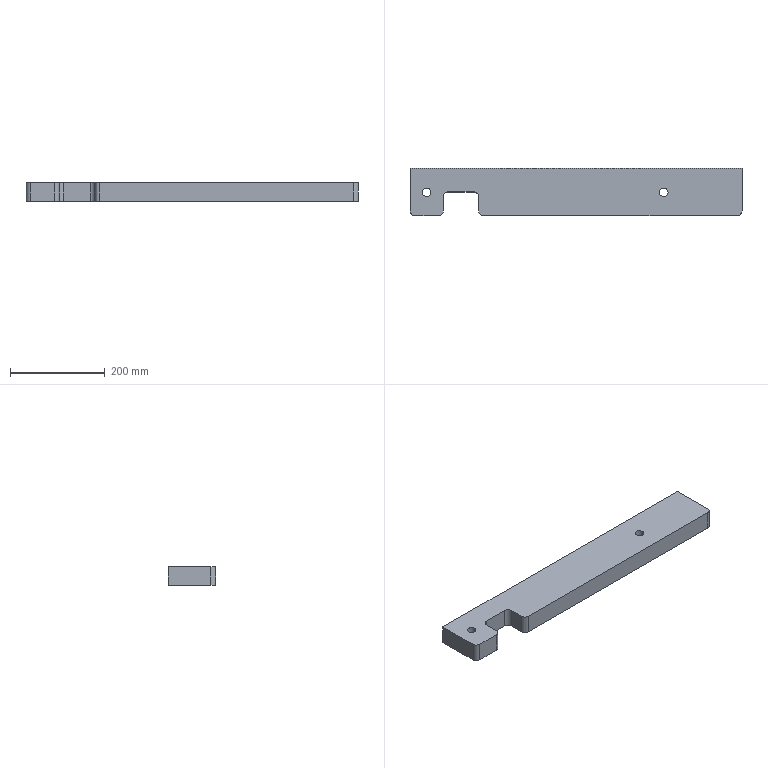Part | SolidWorks | features Extrusion 1, Fillet 1 | 1 solid | 20 faces | box 700 x 100 x 40 mm | volume 2627926 mm3 | cylinder 10 | plane 10 | commonest cylinder face diameters 20 x6 18 x4
STEP:
#1=CARTESIAN_POINT('',(526.,49.,40.));
#2=VERTEX_POINT('',#1);
#3=CARTESIAN_POINT('',(544.,49.,40.));
#4=VERTEX_POINT('',#3);
#5=CARTESIAN_POINT('',(535.,49.,40.));
#6=DIRECTION('',(0.,0.,1.));
#7=DIRECTION('',(1.,0.,0.));
#8=AXIS2_PLACEMENT_3D('',#5,#6,#7);
#9=CIRCLE('',#8,9.);
#10=EDGE_CURVE('',#2,#4,#9,.T.);
#11=ORIENTED_EDGE('',*,*,#10,.T.);
#12=CARTESIAN_POINT('',(544.,49.,0.));
#13=VERTEX_POINT('',#12);
#14=CARTESIAN_POINT('',(544.,49.,40.));
#15=DIRECTION('',(0.,0.,-1.));
#16=VECTOR('',#15,1000.);
#17=LINE('',#14,#16);
#18=EDGE_CURVE('',#4,#13,#17,.T.);
#19=ORIENTED_EDGE('',*,*,#18,.T.);
#20=CARTESIAN_POINT('',(526.,49.,0.));
#21=VERTEX_POINT('',#20);
#22=CARTESIAN_POINT('',(535.,49.,0.));
#23=DIRECTION('',(0.,0.,1.));
#24=DIRECTION('',(1.,0.,0.));
#25=AXIS2_PLACEMENT_3D('',#22,#23,#24);
#26=CIRCLE('',#25,9.);
#27=EDGE_CURVE('',#21,#13,#26,.T.);
#28=ORIENTED_EDGE('',*,*,#27,.F.);
#29=CARTESIAN_POINT('',(526.,49.,40.));
#30=DIRECTION('',(0.,0.,-1.));
#31=VECTOR('',#30,1000.);
#32=LINE('',#29,#31);
#33=EDGE_CURVE('',#2,#21,#32,.T.);
#34=ORIENTED_EDGE('',*,*,#33,.F.);
#35=EDGE_LOOP('',(#11,#19,#28,#34));
#36=FACE_OUTER_BOUND('',#35,.T.);
#37=CARTESIAN_POINT('',(535.,49.,40.));
#38=DIRECTION('',(0.,0.,-1.));
#39=DIRECTION('',(-1.,0.,0.));
#40=AXIS2_PLACEMENT_3D('',#37,#38,#39);
#41=CYLINDRICAL_SURFACE('',#40,9.);
#42=ADVANCED_FACE('',(#36),#41,.F.);
#43=CARTESIAN_POINT('',(26.,49.,40.));
#44=VERTEX_POINT('',#43);
#45=CARTESIAN_POINT('',(44.,49.,40.));
#46=VERTEX_POINT('',#45);
#47=CARTESIAN_POINT('',(35.,49.,40.));
#48=DIRECTION('',(0.,0.,1.));
#49=DIRECTION('',(1.,0.,0.));
#50=AXIS2_PLACEMENT_3D('',#47,#48,#49);
#51=CIRCLE('',#50,9.);
#52=EDGE_CURVE('',#44,#46,#51,.T.);
#53=ORIENTED_EDGE('',*,*,#52,.T.);
#54=CARTESIAN_POINT('',(44.,49.,0.));
#55=VERTEX_POINT('',#54);
#56=CARTESIAN_POINT('',(44.,49.,40.));
#57=DIRECTION('',(0.,0.,-1.));
#58=VECTOR('',#57,1000.);
#59=LINE('',#56,#58);
#60=EDGE_CURVE('',#46,#55,#59,.T.);
#61=ORIENTED_EDGE('',*,*,#60,.T.);
#62=CARTESIAN_POINT('',(26.,49.,0.));
#63=VERTEX_POINT('',#62);
#64=CARTESIAN_POINT('',(35.,49.,0.));
#65=DIRECTION('',(0.,0.,1.));
#66=DIRECTION('',(1.,0.,0.));
#67=AXIS2_PLACEMENT_3D('',#64,#65,#66);
#68=CIRCLE('',#67,9.);
#69=EDGE_CURVE('',#63,#55,#68,.T.);
#70=ORIENTED_EDGE('',*,*,#69,.F.);
#71=CARTESIAN_POINT('',(26.,49.,40.));
#72=DIRECTION('',(0.,0.,-1.));
#73=VECTOR('',#72,1000.);
#74=LINE('',#71,#73);
#75=EDGE_CURVE('',#44,#63,#74,.T.);
#76=ORIENTED_EDGE('',*,*,#75,.F.);
#77=EDGE_LOOP('',(#53,#61,#70,#76));
#78=FACE_OUTER_BOUND('',#77,.T.);
#79=CARTESIAN_POINT('',(35.,49.,40.));
#80=DIRECTION('',(0.,0.,-1.));
#81=DIRECTION('',(-1.,0.,0.));
#82=AXIS2_PLACEMENT_3D('',#79,#80,#81);
#83=CYLINDRICAL_SURFACE('',#82,9.);
#84=ADVANCED_FACE('',(#78),#83,.F.);
#85=ORIENTED_EDGE('',*,*,#52,.F.);
#86=CARTESIAN_POINT('',(35.,49.,40.));
#87=DIRECTION('',(0.,0.,1.));
#88=DIRECTION('',(1.,0.,0.));
#89=AXIS2_PLACEMENT_3D('',#86,#87,#88);
#90=CIRCLE('',#89,9.);
#91=EDGE_CURVE('',#46,#44,#90,.T.);
#92=ORIENTED_EDGE('',*,*,#91,.F.);
#93=EDGE_LOOP('',(#85,#92));
#94=FACE_BOUND('',#93,.T.);
#95=CARTESIAN_POINT('',(155.,0.,40.));
#96=VERTEX_POINT('',#95);
#97=CARTESIAN_POINT('',(690.,0.,40.));
#98=VERTEX_POINT('',#97);
#99=CARTESIAN_POINT('',(700.,0.,40.));
#100=DIRECTION('',(1.,0.,0.));
#101=VECTOR('',#100,1000.);
#102=LINE('',#99,#101);
#103=EDGE_CURVE('',#96,#98,#102,.T.);
#104=ORIENTED_EDGE('',*,*,#103,.T.);
#105=CARTESIAN_POINT('',(700.,10.,40.));
#106=VERTEX_POINT('',#105);
#107=CARTESIAN_POINT('',(690.,10.,40.));
#108=DIRECTION('',(0.,0.,1.));
#109=DIRECTION('',(1.,0.,0.));
#110=AXIS2_PLACEMENT_3D('',#107,#108,#109);
#111=CIRCLE('',#110,10.);
#112=EDGE_CURVE('',#98,#106,#111,.T.);
#113=ORIENTED_EDGE('',*,*,#112,.T.);
#114=CARTESIAN_POINT('',(700.,100.,40.));
#115=VERTEX_POINT('',#114);
#116=CARTESIAN_POINT('',(700.,0.,40.));
#117=DIRECTION('',(0.,1.,0.));
#118=VECTOR('',#117,1000.);
#119=LINE('',#116,#118);
#120=EDGE_CURVE('',#106,#115,#119,.T.);
#121=ORIENTED_EDGE('',*,*,#120,.T.);
#122=CARTESIAN_POINT('',(0.,100.,40.));
#123=VERTEX_POINT('',#122);
#124=CARTESIAN_POINT('',(0.,100.,40.));
#125=DIRECTION('',(-1.,0.,0.));
#126=VECTOR('',#125,1000.);
#127=LINE('',#124,#126);
#128=EDGE_CURVE('',#115,#123,#127,.T.);
#129=ORIENTED_EDGE('',*,*,#128,.T.);
#130=CARTESIAN_POINT('',(0.,10.,40.));
#131=VERTEX_POINT('',#130);
#132=CARTESIAN_POINT('',(0.,0.,40.));
#133=DIRECTION('',(0.,-1.,0.));
#134=VECTOR('',#133,1000.);
#135=LINE('',#132,#134);
#136=EDGE_CURVE('',#123,#131,#135,.T.);
#137=ORIENTED_EDGE('',*,*,#136,.T.);
#138=CARTESIAN_POINT('',(10.,0.,40.));
#139=VERTEX_POINT('',#138);
#140=CARTESIAN_POINT('',(10.,10.,40.));
#141=DIRECTION('',(0.,0.,1.));
#142=DIRECTION('',(1.,0.,0.));
#143=AXIS2_PLACEMENT_3D('',#140,#141,#142);
#144=CIRCLE('',#143,10.);
#145=EDGE_CURVE('',#131,#139,#144,.T.);
#146=ORIENTED_EDGE('',*,*,#145,.T.);
#147=CARTESIAN_POINT('',(60.,0.,40.));
#148=VERTEX_POINT('',#147);
#149=CARTESIAN_POINT('',(70.,0.,40.));
#150=DIRECTION('',(1.,0.,0.));
#151=VECTOR('',#150,1000.);
#152=LINE('',#149,#151);
#153=EDGE_CURVE('',#139,#148,#152,.T.);
#154=ORIENTED_EDGE('',*,*,#153,.T.);
#155=CARTESIAN_POINT('',(70.,10.,40.));
#156=VERTEX_POINT('',#155);
#157=CARTESIAN_POINT('',(60.,10.,40.));
#158=DIRECTION('',(0.,0.,1.));
#159=DIRECTION('',(1.,0.,0.));
#160=AXIS2_PLACEMENT_3D('',#157,#158,#159);
#161=CIRCLE('',#160,10.);
#162=EDGE_CURVE('',#148,#156,#161,.T.);
#163=ORIENTED_EDGE('',*,*,#162,.T.);
#164=CARTESIAN_POINT('',(70.,40.,40.));
#165=VERTEX_POINT('',#164);
#166=CARTESIAN_POINT('',(70.,0.,40.));
#167=DIRECTION('',(0.,1.,0.));
#168=VECTOR('',#167,1000.);
#169=LINE('',#166,#168);
#170=EDGE_CURVE('',#156,#165,#169,.T.);
#171=ORIENTED_EDGE('',*,*,#170,.T.);
#172=CARTESIAN_POINT('',(80.,50.,40.));
#173=VERTEX_POINT('',#172);
#174=CARTESIAN_POINT('',(80.,40.,40.));
#175=DIRECTION('',(0.,0.,-1.));
#176=DIRECTION('',(1.,0.,0.));
#177=AXIS2_PLACEMENT_3D('',#174,#175,#176);
#178=CIRCLE('',#177,10.);
#179=EDGE_CURVE('',#165,#173,#178,.T.);
#180=ORIENTED_EDGE('',*,*,#179,.T.);
#181=CARTESIAN_POINT('',(135.,50.,40.));
#182=VERTEX_POINT('',#181);
#183=CARTESIAN_POINT('',(70.,50.,40.));
#184=DIRECTION('',(1.,0.,0.));
#185=VECTOR('',#184,1000.);
#186=LINE('',#183,#185);
#187=EDGE_CURVE('',#173,#182,#186,.T.);
#188=ORIENTED_EDGE('',*,*,#187,.T.);
#189=CARTESIAN_POINT('',(145.,40.,40.));
#190=VERTEX_POINT('',#189);
#191=CARTESIAN_POINT('',(135.,40.,40.));
#192=DIRECTION('',(0.,0.,-1.));
#193=DIRECTION('',(1.,0.,0.));
#194=AXIS2_PLACEMENT_3D('',#191,#192,#193);
#195=CIRCLE('',#194,10.);
#196=EDGE_CURVE('',#182,#190,#195,.T.);
#197=ORIENTED_EDGE('',*,*,#196,.T.);
#198=CARTESIAN_POINT('',(145.,10.,40.));
#199=VERTEX_POINT('',#198);
#200=CARTESIAN_POINT('',(145.,50.,40.));
#201=DIRECTION('',(0.,-1.,0.));
#202=VECTOR('',#201,1000.);
#203=LINE('',#200,#202);
#204=EDGE_CURVE('',#190,#199,#203,.T.);
#205=ORIENTED_EDGE('',*,*,#204,.T.);
#206=CARTESIAN_POINT('',(155.,10.,40.));
#207=DIRECTION('',(0.,0.,1.));
#208=DIRECTION('',(1.,0.,0.));
#209=AXIS2_PLACEMENT_3D('',#206,#207,#208);
#210=CIRCLE('',#209,10.);
#211=EDGE_CURVE('',#199,#96,#210,.T.);
#212=ORIENTED_EDGE('',*,*,#211,.T.);
#213=EDGE_LOOP('',(#104,#113,#121,#129,#137,#146,#154,#163,#171,#180,#188,#197,#205,#212));
#214=FACE_OUTER_BOUND('',#213,.T.);
#215=ORIENTED_EDGE('',*,*,#10,.F.);
#216=CARTESIAN_POINT('',(535.,49.,40.));
#217=DIRECTION('',(0.,0.,1.));
#218=DIRECTION('',(1.,0.,0.));
#219=AXIS2_PLACEMENT_3D('',#216,#217,#218);
#220=CIRCLE('',#219,9.);
#221=EDGE_CURVE('',#4,#2,#220,.T.);
#222=ORIENTED_EDGE('',*,*,#221,.F.);
#223=EDGE_LOOP('',(#215,#222));
#224=FACE_BOUND('',#223,.T.);
#225=CARTESIAN_POINT('',(0.,0.,40.));
#226=DIRECTION('',(0.,0.,1.));
#227=DIRECTION('',(1.,0.,0.));
#228=AXIS2_PLACEMENT_3D('',#225,#226,#227);
#229=PLANE('',#228);
#230=ADVANCED_FACE('',(#94,#214,#224),#229,.T.);
#231=CARTESIAN_POINT('',(700.,10.,0.));
#232=VERTEX_POINT('',#231);
#233=CARTESIAN_POINT('',(700.,100.,0.));
#234=VERTEX_POINT('',#233);
#235=CARTESIAN_POINT('',(700.,0.,0.));
#236=DIRECTION('',(0.,1.,0.));
#237=VECTOR('',#236,1000.);
#238=LINE('',#235,#237);
#239=EDGE_CURVE('',#232,#234,#238,.T.);
#240=ORIENTED_EDGE('',*,*,#239,.F.);
#241=CARTESIAN_POINT('',(690.,0.,0.));
#242=VERTEX_POINT('',#241);
#243=CARTESIAN_POINT('',(690.,10.,0.));
#244=DIRECTION('',(0.,0.,-1.));
#245=DIRECTION('',(1.,0.,0.));
#246=AXIS2_PLACEMENT_3D('',#243,#244,#245);
#247=CIRCLE('',#246,10.);
#248=EDGE_CURVE('',#232,#242,#247,.T.);
#249=ORIENTED_EDGE('',*,*,#248,.T.);
#250=CARTESIAN_POINT('',(155.,0.,0.));
#251=VERTEX_POINT('',#250);
#252=CARTESIAN_POINT('',(700.,0.,0.));
#253=DIRECTION('',(1.,0.,0.));
#254=VECTOR('',#253,1000.);
#255=LINE('',#252,#254);
#256=EDGE_CURVE('',#251,#242,#255,.T.);
#257=ORIENTED_EDGE('',*,*,#256,.F.);
#258=CARTESIAN_POINT('',(145.,10.,0.));
#259=VERTEX_POINT('',#258);
#260=CARTESIAN_POINT('',(155.,10.,0.));
#261=DIRECTION('',(0.,0.,-1.));
#262=DIRECTION('',(1.,0.,0.));
#263=AXIS2_PLACEMENT_3D('',#260,#261,#262);
#264=CIRCLE('',#263,10.);
#265=EDGE_CURVE('',#251,#259,#264,.T.);
#266=ORIENTED_EDGE('',*,*,#265,.T.);
#267=CARTESIAN_POINT('',(145.,40.,0.));
#268=VERTEX_POINT('',#267);
#269=CARTESIAN_POINT('',(145.,50.,0.));
#270=DIRECTION('',(0.,-1.,0.));
#271=VECTOR('',#270,1000.);
#272=LINE('',#269,#271);
#273=EDGE_CURVE('',#268,#259,#272,.T.);
#274=ORIENTED_EDGE('',*,*,#273,.F.);
#275=CARTESIAN_POINT('',(135.,50.,0.));
#276=VERTEX_POINT('',#275);
#277=CARTESIAN_POINT('',(135.,40.,0.));
#278=DIRECTION('',(0.,0.,1.));
#279=DIRECTION('',(1.,0.,0.));
#280=AXIS2_PLACEMENT_3D('',#277,#278,#279);
#281=CIRCLE('',#280,10.);
#282=EDGE_CURVE('',#268,#276,#281,.T.);
#283=ORIENTED_EDGE('',*,*,#282,.T.);
#284=CARTESIAN_POINT('',(80.,50.,0.));
#285=VERTEX_POINT('',#284);
#286=CARTESIAN_POINT('',(70.,50.,0.));
#287=DIRECTION('',(1.,0.,0.));
#288=VECTOR('',#287,1000.);
#289=LINE('',#286,#288);
#290=EDGE_CURVE('',#285,#276,#289,.T.);
#291=ORIENTED_EDGE('',*,*,#290,.F.);
#292=CARTESIAN_POINT('',(70.,40.,0.));
#293=VERTEX_POINT('',#292);
#294=CARTESIAN_POINT('',(80.,40.,0.));
#295=DIRECTION('',(0.,0.,1.));
#296=DIRECTION('',(1.,0.,0.));
#297=AXIS2_PLACEMENT_3D('',#294,#295,#296);
#298=CIRCLE('',#297,10.);
#299=EDGE_CURVE('',#285,#293,#298,.T.);
#300=ORIENTED_EDGE('',*,*,#299,.T.);
#301=CARTESIAN_POINT('',(70.,10.,0.));
#302=VERTEX_POINT('',#301);
#303=CARTESIAN_POINT('',(70.,0.,0.));
#304=DIRECTION('',(0.,1.,0.));
#305=VECTOR('',#304,1000.);
#306=LINE('',#303,#305);
#307=EDGE_CURVE('',#302,#293,#306,.T.);
#308=ORIENTED_EDGE('',*,*,#307,.F.);
#309=CARTESIAN_POINT('',(60.,0.,0.));
#310=VERTEX_POINT('',#309);
#311=CARTESIAN_POINT('',(60.,10.,0.));
#312=DIRECTION('',(0.,0.,-1.));
#313=DIRECTION('',(1.,0.,0.));
#314=AXIS2_PLACEMENT_3D('',#311,#312,#313);
#315=CIRCLE('',#314,10.);
#316=EDGE_CURVE('',#302,#310,#315,.T.);
#317=ORIENTED_EDGE('',*,*,#316,.T.);
#318=CARTESIAN_POINT('',(10.,0.,0.));
#319=VERTEX_POINT('',#318);
#320=CARTESIAN_POINT('',(70.,0.,0.));
#321=DIRECTION('',(1.,0.,0.));
#322=VECTOR('',#321,1000.);
#323=LINE('',#320,#322);
#324=EDGE_CURVE('',#319,#310,#323,.T.);
#325=ORIENTED_EDGE('',*,*,#324,.F.);
#326=CARTESIAN_POINT('',(0.,10.,0.));
#327=VERTEX_POINT('',#326);
#328=CARTESIAN_POINT('',(10.,10.,0.));
#329=DIRECTION('',(0.,0.,-1.));
#330=DIRECTION('',(1.,0.,0.));
#331=AXIS2_PLACEMENT_3D('',#328,#329,#330);
#332=CIRCLE('',#331,10.);
#333=EDGE_CURVE('',#319,#327,#332,.T.);
#334=ORIENTED_EDGE('',*,*,#333,.T.);
#335=CARTESIAN_POINT('',(0.,100.,0.));
#336=VERTEX_POINT('',#335);
#337=CARTESIAN_POINT('',(0.,0.,0.));
#338=DIRECTION('',(0.,-1.,0.));
#339=VECTOR('',#338,1000.);
#340=LINE('',#337,#339);
#341=EDGE_CURVE('',#336,#327,#340,.T.);
#342=ORIENTED_EDGE('',*,*,#341,.F.);
#343=CARTESIAN_POINT('',(0.,100.,0.));
#344=DIRECTION('',(-1.,0.,0.));
#345=VECTOR('',#344,1000.);
#346=LINE('',#343,#345);
#347=EDGE_CURVE('',#234,#336,#346,.T.);
#348=ORIENTED_EDGE('',*,*,#347,.F.);
#349=EDGE_LOOP('',(#240,#249,#257,#266,#274,#283,#291,#300,#308,#317,#325,#334,#342,#348));
#350=FACE_OUTER_BOUND('',#349,.T.);
#351=ORIENTED_EDGE('',*,*,#69,.T.);
#352=CARTESIAN_POINT('',(35.,49.,0.));
#353=DIRECTION('',(0.,0.,1.));
#354=DIRECTION('',(1.,0.,0.));
#355=AXIS2_PLACEMENT_3D('',#352,#353,#354);
#356=CIRCLE('',#355,9.);
#357=EDGE_CURVE('',#55,#63,#356,.T.);
#358=ORIENTED_EDGE('',*,*,#357,.T.);
#359=EDGE_LOOP('',(#351,#358));
#360=FACE_BOUND('',#359,.T.);
#361=ORIENTED_EDGE('',*,*,#27,.T.);
#362=CARTESIAN_POINT('',(535.,49.,0.));
#363=DIRECTION('',(0.,0.,1.));
#364=DIRECTION('',(1.,0.,0.));
#365=AXIS2_PLACEMENT_3D('',#362,#363,#364);
#366=CIRCLE('',#365,9.);
#367=EDGE_CURVE('',#13,#21,#366,.T.);
#368=ORIENTED_EDGE('',*,*,#367,.T.);
#369=EDGE_LOOP('',(#361,#368));
#370=FACE_BOUND('',#369,.T.);
#371=CARTESIAN_POINT('',(0.,0.,0.));
#372=DIRECTION('',(0.,0.,1.));
#373=DIRECTION('',(1.,0.,0.));
#374=AXIS2_PLACEMENT_3D('',#371,#372,#373);
#375=PLANE('',#374);
#376=ADVANCED_FACE('',(#350,#360,#370),#375,.F.);
#377=ORIENTED_EDGE('',*,*,#256,.T.);
#378=CARTESIAN_POINT('',(690.,0.,40.));
#379=DIRECTION('',(0.,0.,1.));
#380=VECTOR('',#379,1000.);
#381=LINE('',#378,#380);
#382=EDGE_CURVE('',#242,#98,#381,.T.);
#383=ORIENTED_EDGE('',*,*,#382,.T.);
#384=ORIENTED_EDGE('',*,*,#103,.F.);
#385=CARTESIAN_POINT('',(155.,0.,40.));
#386=DIRECTION('',(0.,0.,-1.));
#387=VECTOR('',#386,1000.);
#388=LINE('',#385,#387);
#389=EDGE_CURVE('',#96,#251,#388,.T.);
#390=ORIENTED_EDGE('',*,*,#389,.T.);
#391=EDGE_LOOP('',(#377,#383,#384,#390));
#392=FACE_OUTER_BOUND('',#391,.T.);
#393=CARTESIAN_POINT('',(700.,0.,40.));
#394=DIRECTION('',(0.,1.,0.));
#395=DIRECTION('',(-1.,0.,0.));
#396=AXIS2_PLACEMENT_3D('',#393,#394,#395);
#397=PLANE('',#396);
#398=ADVANCED_FACE('',(#392),#397,.F.);
#399=ORIENTED_EDGE('',*,*,#120,.F.);
#400=CARTESIAN_POINT('',(700.,10.,40.));
#401=DIRECTION('',(0.,0.,-1.));
#402=VECTOR('',#401,1000.);
#403=LINE('',#400,#402);
#404=EDGE_CURVE('',#106,#232,#403,.T.);
#405=ORIENTED_EDGE('',*,*,#404,.T.);
#406=ORIENTED_EDGE('',*,*,#239,.T.);
#407=CARTESIAN_POINT('',(700.,100.,40.));
#408=DIRECTION('',(0.,0.,-1.));
#409=VECTOR('',#408,1000.);
#410=LINE('',#407,#409);
#411=EDGE_CURVE('',#115,#234,#410,.T.);
#412=ORIENTED_EDGE('',*,*,#411,.F.);
#413=EDGE_LOOP('',(#399,#405,#406,#412));
#414=FACE_OUTER_BOUND('',#413,.T.);
#415=CARTESIAN_POINT('',(700.,0.,40.));
#416=DIRECTION('',(-1.,0.,0.));
#417=DIRECTION('',(0.,0.,1.));
#418=AXIS2_PLACEMENT_3D('',#415,#416,#417);
#419=PLANE('',#418);
#420=ADVANCED_FACE('',(#414),#419,.F.);
#421=ORIENTED_EDGE('',*,*,#347,.T.);
#422=CARTESIAN_POINT('',(0.,100.,40.));
#423=DIRECTION('',(0.,0.,-1.));
#424=VECTOR('',#423,1000.);
#425=LINE('',#422,#424);
#426=EDGE_CURVE('',#123,#336,#425,.T.);
#427=ORIENTED_EDGE('',*,*,#426,.F.);
#428=ORIENTED_EDGE('',*,*,#128,.F.);
#429=ORIENTED_EDGE('',*,*,#411,.T.);
#430=EDGE_LOOP('',(#421,#427,#428,#429));
#431=FACE_OUTER_BOUND('',#430,.T.);
#432=CARTESIAN_POINT('',(0.,100.,40.));
#433=DIRECTION('',(0.,-1.,0.));
#434=DIRECTION('',(1.,0.,0.));
#435=AXIS2_PLACEMENT_3D('',#432,#433,#434);
#436=PLANE('',#435);
#437=ADVANCED_FACE('',(#431),#436,.F.);
#438=ORIENTED_EDGE('',*,*,#341,.T.);
#439=CARTESIAN_POINT('',(0.,10.,40.));
#440=DIRECTION('',(0.,0.,1.));
#441=VECTOR('',#440,1000.);
#442=LINE('',#439,#441);
#443=EDGE_CURVE('',#327,#131,#442,.T.);
#444=ORIENTED_EDGE('',*,*,#443,.T.);
#445=ORIENTED_EDGE('',*,*,#136,.F.);
#446=ORIENTED_EDGE('',*,*,#426,.T.);
#447=EDGE_LOOP('',(#438,#444,#445,#446));
#448=FACE_OUTER_BOUND('',#447,.T.);
#449=CARTESIAN_POINT('',(0.,0.,40.));
#450=DIRECTION('',(1.,0.,0.));
#451=DIRECTION('',(0.,0.,-1.));
#452=AXIS2_PLACEMENT_3D('',#449,#450,#451);
#453=PLANE('',#452);
#454=ADVANCED_FACE('',(#448),#453,.F.);
#455=ORIENTED_EDGE('',*,*,#153,.F.);
#456=CARTESIAN_POINT('',(10.,0.,40.));
#457=DIRECTION('',(0.,0.,-1.));
#458=VECTOR('',#457,1000.);
#459=LINE('',#456,#458);
#460=EDGE_CURVE('',#139,#319,#459,.T.);
#461=ORIENTED_EDGE('',*,*,#460,.T.);
#462=ORIENTED_EDGE('',*,*,#324,.T.);
#463=CARTESIAN_POINT('',(60.,0.,40.));
#464=DIRECTION('',(0.,0.,1.));
#465=VECTOR('',#464,1000.);
#466=LINE('',#463,#465);
#467=EDGE_CURVE('',#310,#148,#466,.T.);
#468=ORIENTED_EDGE('',*,*,#467,.T.);
#469=EDGE_LOOP('',(#455,#461,#462,#468));
#470=FACE_OUTER_BOUND('',#469,.T.);
#471=CARTESIAN_POINT('',(70.,0.,40.));
#472=DIRECTION('',(0.,1.,0.));
#473=DIRECTION('',(-1.,0.,0.));
#474=AXIS2_PLACEMENT_3D('',#471,#472,#473);
#475=PLANE('',#474);
#476=ADVANCED_FACE('',(#470),#475,.F.);
#477=ORIENTED_EDGE('',*,*,#170,.F.);
#478=CARTESIAN_POINT('',(70.,10.,40.));
#479=DIRECTION('',(0.,0.,-1.));
#480=VECTOR('',#479,1000.);
#481=LINE('',#478,#480);
#482=EDGE_CURVE('',#156,#302,#481,.T.);
#483=ORIENTED_EDGE('',*,*,#482,.T.);
#484=ORIENTED_EDGE('',*,*,#307,.T.);
#485=CARTESIAN_POINT('',(70.,40.,40.));
#486=DIRECTION('',(0.,0.,1.));
#487=VECTOR('',#486,1000.);
#488=LINE('',#485,#487);
#489=EDGE_CURVE('',#293,#165,#488,.T.);
#490=ORIENTED_EDGE('',*,*,#489,.T.);
#491=EDGE_LOOP('',(#477,#483,#484,#490));
#492=FACE_OUTER_BOUND('',#491,.T.);
#493=CARTESIAN_POINT('',(70.,0.,40.));
#494=DIRECTION('',(-1.,0.,0.));
#495=DIRECTION('',(0.,0.,1.));
#496=AXIS2_PLACEMENT_3D('',#493,#494,#495);
#497=PLANE('',#496);
#498=ADVANCED_FACE('',(#492),#497,.F.);
#499=ORIENTED_EDGE('',*,*,#187,.F.);
#500=CARTESIAN_POINT('',(80.,50.,0.));
#501=DIRECTION('',(0.,0.,-1.));
#502=VECTOR('',#501,1000.);
#503=LINE('',#500,#502);
#504=EDGE_CURVE('',#173,#285,#503,.T.);
#505=ORIENTED_EDGE('',*,*,#504,.T.);
#506=ORIENTED_EDGE('',*,*,#290,.T.);
#507=CARTESIAN_POINT('',(135.,50.,40.));
#508=DIRECTION('',(0.,0.,1.));
#509=VECTOR('',#508,1000.);
#510=LINE('',#507,#509);
#511=EDGE_CURVE('',#276,#182,#510,.T.);
#512=ORIENTED_EDGE('',*,*,#511,.T.);
#513=EDGE_LOOP('',(#499,#505,#506,#512));
#514=FACE_OUTER_BOUND('',#513,.T.);
#515=CARTESIAN_POINT('',(70.,50.,40.));
#516=DIRECTION('',(0.,1.,0.));
#517=DIRECTION('',(0.,0.,1.));
#518=AXIS2_PLACEMENT_3D('',#515,#516,#517);
#519=PLANE('',#518);
#520=ADVANCED_FACE('',(#514),#519,.F.);
#521=ORIENTED_EDGE('',*,*,#273,.T.);
#522=CARTESIAN_POINT('',(145.,10.,40.));
#523=DIRECTION('',(0.,0.,1.));
#524=VECTOR('',#523,1000.);
#525=LINE('',#522,#524);
#526=EDGE_CURVE('',#259,#199,#525,.T.);
#527=ORIENTED_EDGE('',*,*,#526,.T.);
#528=ORIENTED_EDGE('',*,*,#204,.F.);
#529=CARTESIAN_POINT('',(145.,40.,0.));
#530=DIRECTION('',(0.,0.,-1.));
#531=VECTOR('',#530,1000.);
#532=LINE('',#529,#531);
#533=EDGE_CURVE('',#190,#268,#532,.T.);
#534=ORIENTED_EDGE('',*,*,#533,.T.);
#535=EDGE_LOOP('',(#521,#527,#528,#534));
#536=FACE_OUTER_BOUND('',#535,.T.);
#537=CARTESIAN_POINT('',(145.,50.,40.));
#538=DIRECTION('',(1.,0.,0.));
#539=DIRECTION('',(0.,0.,-1.));
#540=AXIS2_PLACEMENT_3D('',#537,#538,#539);
#541=PLANE('',#540);
#542=ADVANCED_FACE('',(#536),#541,.F.);
#543=ORIENTED_EDGE('',*,*,#60,.F.);
#544=ORIENTED_EDGE('',*,*,#91,.T.);
#545=ORIENTED_EDGE('',*,*,#75,.T.);
#546=ORIENTED_EDGE('',*,*,#357,.F.);
#547=EDGE_LOOP('',(#543,#544,#545,#546));
#548=FACE_OUTER_BOUND('',#547,.T.);
#549=CARTESIAN_POINT('',(35.,49.,40.));
#550=DIRECTION('',(0.,0.,-1.));
#551=DIRECTION('',(-1.,0.,0.));
#552=AXIS2_PLACEMENT_3D('',#549,#550,#551);
#553=CYLINDRICAL_SURFACE('',#552,9.);
#554=ADVANCED_FACE('',(#548),#553,.F.);
#555=ORIENTED_EDGE('',*,*,#18,.F.);
#556=ORIENTED_EDGE('',*,*,#221,.T.);
#557=ORIENTED_EDGE('',*,*,#33,.T.);
#558=ORIENTED_EDGE('',*,*,#367,.F.);
#559=EDGE_LOOP('',(#555,#556,#557,#558));
#560=FACE_OUTER_BOUND('',#559,.T.);
#561=CARTESIAN_POINT('',(535.,49.,40.));
#562=DIRECTION('',(0.,0.,-1.));
#563=DIRECTION('',(-1.,0.,0.));
#564=AXIS2_PLACEMENT_3D('',#561,#562,#563);
#565=CYLINDRICAL_SURFACE('',#564,9.);
#566=ADVANCED_FACE('',(#560),#565,.F.);
#567=ORIENTED_EDGE('',*,*,#112,.F.);
#568=ORIENTED_EDGE('',*,*,#382,.F.);
#569=ORIENTED_EDGE('',*,*,#248,.F.);
#570=ORIENTED_EDGE('',*,*,#404,.F.);
#571=EDGE_LOOP('',(#567,#568,#569,#570));
#572=FACE_OUTER_BOUND('',#571,.T.);
#573=CARTESIAN_POINT('',(690.,10.,40.));
#574=DIRECTION('',(0.,0.,-1.));
#575=DIRECTION('',(-1.,0.,0.));
#576=AXIS2_PLACEMENT_3D('',#573,#574,#575);
#577=CYLINDRICAL_SURFACE('',#576,10.);
#578=ADVANCED_FACE('',(#572),#577,.T.);
#579=ORIENTED_EDGE('',*,*,#145,.F.);
#580=ORIENTED_EDGE('',*,*,#443,.F.);
#581=ORIENTED_EDGE('',*,*,#333,.F.);
#582=ORIENTED_EDGE('',*,*,#460,.F.);
#583=EDGE_LOOP('',(#579,#580,#581,#582));
#584=FACE_OUTER_BOUND('',#583,.T.);
#585=CARTESIAN_POINT('',(10.,10.,40.));
#586=DIRECTION('',(0.,0.,-1.));
#587=DIRECTION('',(-1.,0.,0.));
#588=AXIS2_PLACEMENT_3D('',#585,#586,#587);
#589=CYLINDRICAL_SURFACE('',#588,10.);
#590=ADVANCED_FACE('',(#584),#589,.T.);
#591=ORIENTED_EDGE('',*,*,#162,.F.);
#592=ORIENTED_EDGE('',*,*,#467,.F.);
#593=ORIENTED_EDGE('',*,*,#316,.F.);
#594=ORIENTED_EDGE('',*,*,#482,.F.);
#595=EDGE_LOOP('',(#591,#592,#593,#594));
#596=FACE_OUTER_BOUND('',#595,.T.);
#597=CARTESIAN_POINT('',(60.,10.,40.));
#598=DIRECTION('',(0.,0.,-1.));
#599=DIRECTION('',(-1.,0.,0.));
#600=AXIS2_PLACEMENT_3D('',#597,#598,#599);
#601=CYLINDRICAL_SURFACE('',#600,10.);
#602=ADVANCED_FACE('',(#596),#601,.T.);
#603=ORIENTED_EDGE('',*,*,#211,.F.);
#604=ORIENTED_EDGE('',*,*,#526,.F.);
#605=ORIENTED_EDGE('',*,*,#265,.F.);
#606=ORIENTED_EDGE('',*,*,#389,.F.);
#607=EDGE_LOOP('',(#603,#604,#605,#606));
#608=FACE_OUTER_BOUND('',#607,.T.);
#609=CARTESIAN_POINT('',(155.,10.,40.));
#610=DIRECTION('',(0.,0.,-1.));
#611=DIRECTION('',(-1.,0.,0.));
#612=AXIS2_PLACEMENT_3D('',#609,#610,#611);
#613=CYLINDRICAL_SURFACE('',#612,10.);
#614=ADVANCED_FACE('',(#608),#613,.T.);
#615=ORIENTED_EDGE('',*,*,#179,.F.);
#616=ORIENTED_EDGE('',*,*,#489,.F.);
#617=ORIENTED_EDGE('',*,*,#299,.F.);
#618=ORIENTED_EDGE('',*,*,#504,.F.);
#619=EDGE_LOOP('',(#615,#616,#617,#618));
#620=FACE_OUTER_BOUND('',#619,.T.);
#621=CARTESIAN_POINT('',(80.,40.,40.));
#622=DIRECTION('',(0.,0.,1.));
#623=DIRECTION('',(1.,0.,0.));
#624=AXIS2_PLACEMENT_3D('',#621,#622,#623);
#625=CYLINDRICAL_SURFACE('',#624,10.);
#626=ADVANCED_FACE('',(#620),#625,.F.);
#627=ORIENTED_EDGE('',*,*,#196,.F.);
#628=ORIENTED_EDGE('',*,*,#511,.F.);
#629=ORIENTED_EDGE('',*,*,#282,.F.);
#630=ORIENTED_EDGE('',*,*,#533,.F.);
#631=EDGE_LOOP('',(#627,#628,#629,#630));
#632=FACE_OUTER_BOUND('',#631,.T.);
#633=CARTESIAN_POINT('',(135.,40.,40.));
#634=DIRECTION('',(0.,0.,1.));
#635=DIRECTION('',(1.,0.,0.));
#636=AXIS2_PLACEMENT_3D('',#633,#634,#635);
#637=CYLINDRICAL_SURFACE('',#636,10.);
#638=ADVANCED_FACE('',(#632),#637,.F.);
#639=CLOSED_SHELL('',(#42,#84,#230,#376,#398,#420,#437,#454,#476,#498,#520,#542,#554,#566,#578,#590,#602,#614,#626,#638));
#640=MANIFOLD_SOLID_BREP('',#639);
#641=CARTESIAN_POINT('',(0.,0.,0.));
#642=DIRECTION('',(0.,0.,1.));
#643=DIRECTION('',(1.,0.,0.));
#644=AXIS2_PLACEMENT_3D('',#641,#642,#643);
#645=(LENGTH_UNIT()NAMED_UNIT(*)SI_UNIT(.MILLI.,.METRE.));
#646=UNCERTAINTY_MEASURE_WITH_UNIT(LENGTH_MEASURE(0.00001),#645,'','');
#647=(NAMED_UNIT(*)PLANE_ANGLE_UNIT()SI_UNIT($,.RADIAN.));
#648=(NAMED_UNIT(*)SI_UNIT($,.STERADIAN.)SOLID_ANGLE_UNIT());
#649=(GEOMETRIC_REPRESENTATION_CONTEXT(3)GLOBAL_UNCERTAINTY_ASSIGNED_CONTEXT((#646))GLOBAL_UNIT_ASSIGNED_CONTEXT((#645,#647,#648))REPRESENTATION_CONTEXT('',''));
#650=ADVANCED_BREP_SHAPE_REPRESENTATION('',(#640,#644),#649);